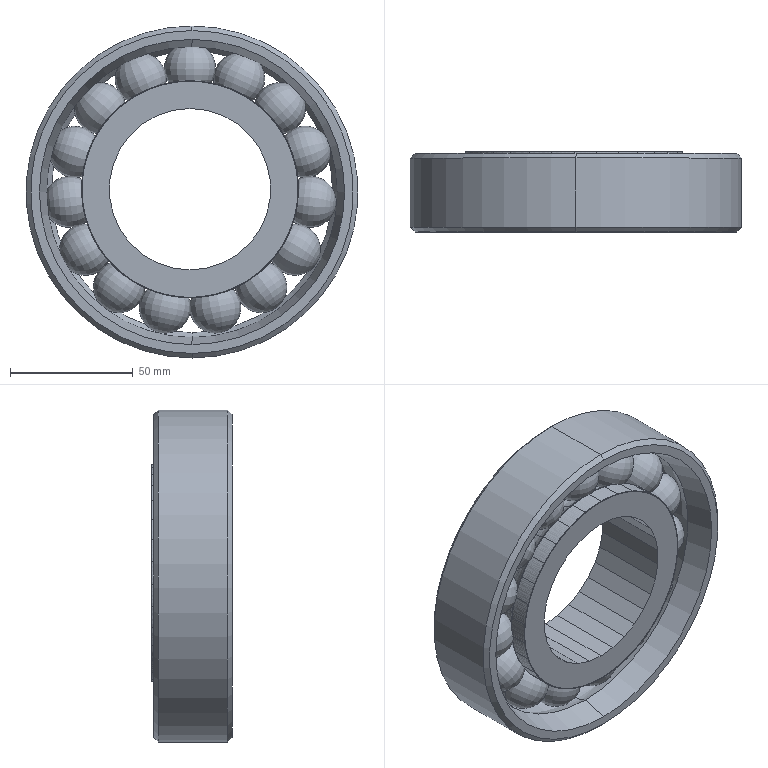Part | SolidWorks | features Revolution 11, Chamfer 1, CirPattern 1, Scale 1 | 16 solids | 254 faces | box 135 x 32.557 x 135 mm | volume 1267368 mm3 | torus 122 | cylinder 94 | plane 32 | cone 6 | commonest cylinder face diameters 88.125 x60 65.625 x30 114.375 x2 135 x2